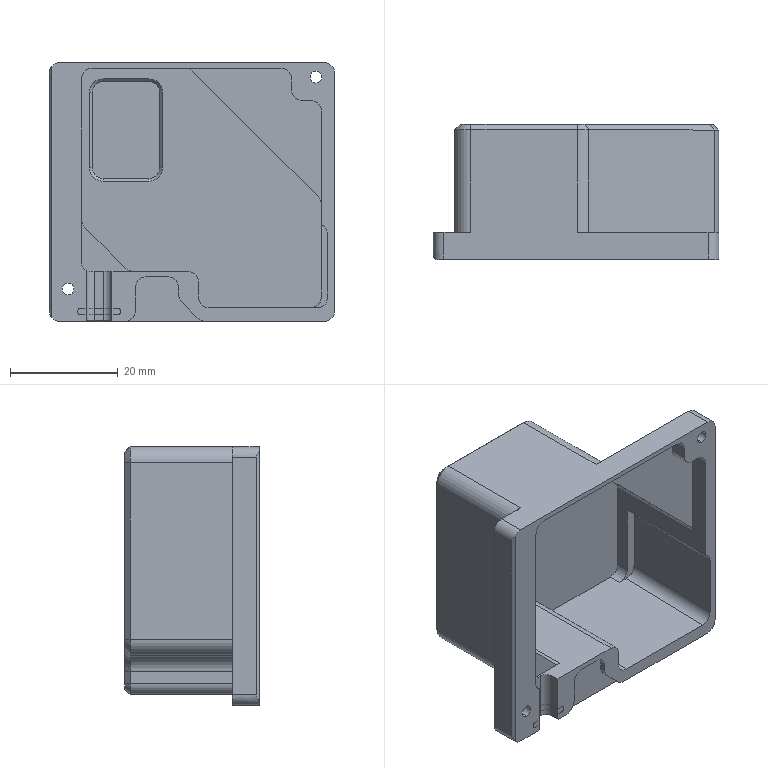NC program | NX | posted with a generic post | part box 53 x 25 x 48 mm
Lines 5523 to 6007 of 6007:
(FLOOR_FACING_1 , TOOL : D4-12-D4-50-3T-FINISH)
N10978 T13 M6
N10980 G54
N10982 G17 G0 G90 X-6.366 Y8.78 B0. C0. S3500 M3
N10984 G43 Z30. H13
N10986 Z-0.3 B-180. C-180.
N10988 G94 G1 Z-3.3 F600.
N10990 X-9.901 Y12.316
N10992 G3 X-11.316 Y12.316 R1.
N10994 G1 X-20.8 Y2.831
N10996 Y16.3
N10998 X-19.
N11000 G3 X-14.8 Y20.5 R4.2
N11002 G1 Y21.8
N11004 X-1.831
N11006 X-11.316 Y12.316
N11008 X-13.437 Y14.437
N11010 X-17.8 Y10.074
N11012 X-18.642 Y8.041
N11014 X-17.8 Y10.074
N11016 Y13.401
N11018 G3 X-12.004 Y18.8 R7.2
N11020 G1 X-9.074
N11022 X-7.041 Y19.642
N11024 X-9.074 Y18.8
N11026 X-13.437 Y14.437
N11028 X-14.144 Y13.73
N11030 G3 X-14.144 Y12.316 R1.
N11032 G1 X-8.487 Y6.659
N11034 Z-0.3
N11036 G0 Z30.
N11038 X29.2 Y-5.243
N11040 Z2.
N11042 G1 Z-1.
N11044 X24.2
N11046 G3 X23.2 Y-6.243 R1.
N11048 G1 Y-8.475
N11050 G3 X22. Y-8.3 R4.2
N11052 G1 X17.95
N11054 Y-4.7
N11056 X18.972
N11058 G3 X21.941 Y-3.47 R4.2
N11060 G1 X23.2 Y-2.211
N11062 Y-6.243
N11064 X21.4
N11066 Y-6.5
N11068 X19.75
N11070 Y-6.449
N11072 G3 X21.4 Y-5.987 R6.
N11074 G1 Y-6.243
N11076 Y-6.5
N11078 X20.657
N11080 G3 X19.657 Y-7.5 R1.
N11082 G1 X29.2
N11084 Z2.
N11086 G0 Z30.
N11088 X5.991 Y-13.155
N11090 Z2.
N11092 G1 Z-1.
N11094 X9.526 Y-16.691
N11096 G3 X10.941 Y-16.691 R1.
N11098 G1 X12.55 Y-15.081
N11100 Y-17.05
N11102 X13.95
N11104 Y-17.549
N11106 G3 X12.865 Y-18.3 R2.2
N11108 G1 X9.331
N11110 X10.941 Y-16.691
N11112 X11.648 Y-15.984
N11114 G3 X11.648 Y-14.569 R1.
N11116 G1 X8.112 Y-11.034
N11118 Z2.
N11120 G0 Z30.
N11122 X5.991 Y-13.155
N11124 Z-0.3
N11126 G1 Z-3.3
N11128 X9.526 Y-16.691
N11130 G3 X10.941 Y-16.691 R1.
N11132 G1 X12.55 Y-15.081
N11134 Y-18.3
N11136 X9.331
N11138 X10.941 Y-16.691
N11140 X11.648 Y-15.984
N11142 G3 X11.648 Y-14.569 R1.
N11144 G1 X8.112 Y-11.034
N11146 Z-0.3
N11148 G0 Z30.
(PLANAR_MILL_7 , TOOL : D4-12-D4-50-3T-FINISH)
N11150 X8.259 Y12.2
N11152 Z-22.
N11154 G1 X6.388 Z-22.098
N11156 X-5.781 Y0.031 Z-23.
N11158 X-2.387 Y-3.363
N11160 X-2.924 Y-3.9
N11162 X-1.85
N11164 Y-2.826
N11166 X-2.387 Y-3.363
N11168 X-4.084 Y-1.666
N11170 X-8.718 Y-6.3
N11172 X0.118
N11174 X0.55 Y-5.868
N11176 Y-0.8
N11178 G2 X1.15 Y3.568 R16.2
N11180 G1 X-4.084 Y-1.666
N11182 X-5.781 Y0.031
N11184 X-11.2 Y-5.388
N11186 Y-8.7
N11188 X1.112
N11190 X2.95 Y-6.862
N11192 Y-0.8
N11194 G2 X9.7 Y11.063 R13.8
N11196 G1 Y12.2
N11198 X6.388
N11200 X-5.781 Y0.031
N11202 X-7.478 Y1.728
N11204 X-13.6 Y-4.394
N11206 Y-11.1
N11208 X2.106
N11210 X5.35 Y-7.856
N11212 Y-0.8
N11214 G2 X12.1 Y9.609 R11.4
N11216 G1 Y14.6
N11218 X5.394
N11220 X-7.478 Y1.728
N11222 X-9.175 Y3.425
N11224 X-16. Y-3.399
N11226 Y-13.5
N11228 X3.101
N11230 X7.75 Y-8.851
N11232 Y-0.8
N11234 G2 X14.5 Y7.914 R9.
N11236 G1 Y17.
N11238 X4.399
N11240 X-9.175 Y3.425
N11242 X-10.872 Y5.122
N11244 X-18.4 Y-2.405
N11246 Y-15.9
N11248 X4.095
N11250 X10.15 Y-9.845
N11252 Y-0.8
N11254 G2 X16.75 Y5.8 R6.6
N11256 G1 X16.9
N11258 Y19.4
N11260 X3.405
N11262 X-10.872 Y5.122
N11264 X-12.569 Y6.819
N11266 X-20.8 Y-1.411
N11268 Y-18.3
N11270 X5.089
N11272 X12.55 Y-10.839
N11274 Y-0.8
N11276 G2 X16.75 Y3.4 R4.2
N11278 G1 X19.3
N11280 Y21.8
N11282 X2.411
N11284 X-12.569 Y6.819
N11286 Z-22.
N11288 G0 Z30.
(FLOOR_FACING_1_COPY , TOOL : D4-12-D4-50-3T-FINISH)
N11290 X-8.481 Y-8.1
N11292 Z-23.
N11294 G1 X-4.6 Z-23.203
N11296 Y-16.4 Z-23.638
N11298 X-11.5 Z-24.
N11300 X-18.4
N11302 Y-8.1
N11304 X-4.6
N11306 Y-16.4
N11308 X-11.5
N11310 Y-13.4
N11312 X-15.4
N11314 Y-11.1
N11316 X-7.6
N11318 Y-13.4
N11320 X-11.5
N11322 X-12.5
N11324 Z-23.
N11326 G0 Z30.
(PLANAR_MILL_7_COPY , TOOL : D4-12-D4-50-3T-FINISH)
N11328 X17.5 Y5.2
N11330 Z-5.66
N11332 G1 Z-7.66
N11334 G3 X19.5 Y3.2 R2.
N11336 G1 Y22.
N11338 X2.328
N11340 X-21. Y-1.328
N11342 Y-18.5
N11344 X5.172
N11346 X12.75 Y-10.922
N11348 Y-0.8
N11350 G2 X16.75 Y3.2 R4.
N11352 G1 X19.5
N11354 G3 X17.5 Y5.2 R2.
N11356 X19.5 Y3.2 R2.
N11358 G1 Y22.
N11360 X2.328
N11362 X-21. Y-1.328
N11364 Y-18.5
N11366 X5.172
N11368 X12.75 Y-10.922
N11370 Y-0.8
N11372 G2 X16.75 Y3.2 R4.
N11374 G1 X19.5
N11376 G3 X17.5 Y5.2 R2.
N11378 G1 Z-5.66
N11380 G0 Z30.
N11382 Z-13.32
N11384 G1 Z-15.32
N11386 G3 X19.5 Y3.2 R2.
N11388 G1 Y22.
N11390 X2.328
N11392 X-21. Y-1.328
N11394 Y-18.5
N11396 X5.172
N11398 X12.75 Y-10.922
N11400 Y-0.8
N11402 G2 X16.75 Y3.2 R4.
N11404 G1 X19.5
N11406 G3 X17.5 Y5.2 R2.
N11408 X19.5 Y3.2 R2.
N11410 G1 Y22.
N11412 X2.328
N11414 X-21. Y-1.328
N11416 Y-18.5
N11418 X5.172
N11420 X12.75 Y-10.922
N11422 Y-0.8
N11424 G2 X16.75 Y3.2 R4.
N11426 G1 X19.5
N11428 G3 X17.5 Y5.2 R2.
N11430 G1 Z-13.32
N11432 G0 Z30.
N11434 Z-20.98
N11436 G1 Z-22.98
N11438 G3 X19.5 Y3.2 R2.
N11440 G1 Y22.
N11442 X2.328
N11444 X-21. Y-1.328
N11446 Y-18.5
N11448 X5.172
N11450 X12.75 Y-10.922
N11452 Y-0.8
N11454 G2 X16.75 Y3.2 R4.
N11456 G1 X19.5
N11458 G3 X17.5 Y5.2 R2.
N11460 X19.5 Y3.2 R2.
N11462 G1 Y22.
N11464 X2.328
N11466 X-21. Y-1.328
N11468 Y-18.5
N11470 X5.172
N11472 X12.75 Y-10.922
N11474 Y-0.8
N11476 G2 X16.75 Y3.2 R4.
N11478 G1 X19.5
N11480 G3 X17.5 Y5.2 R2.
N11482 G1 Z-20.98
N11484 G0 Z30.
(PLANAR_MILL_7_COPY_COPY , TOOL : D4-12-D4-50-3T-FINISH)
N11486 X-6.5 Y-10.
N11488 Z-22.
N11490 G1 Z-24.
N11492 G3 X-4.5 Y-8. R2.
N11494 G1 X-18.5
N11496 Y-16.5
N11498 X-4.5
N11500 Y-8.
N11502 G3 X-6.5 Y-10. R2.
N11504 X-4.5 Y-8. R2.
N11506 G1 X-18.5
N11508 Y-16.5
N11510 X-4.5
N11512 Y-8.
N11514 G3 X-6.5 Y-10. R2.
N11516 G1 Z-22.
N11518 G0 Z30.
(PLANAR_MILL_7_COPY_COPY_COPY , TOOL : D4-12-D4-50-3T-FINISH)
N11520 X4.328 Y20.
N11522 Z-1.3
N11524 G1 Z-3.3
N11526 G3 X2.328 Y22. R2.
N11528 G1 X-15.
N11530 Y20.5
N11532 G2 X-19. Y16.5 R4.
N11534 G1 X-20.95
N11536 Y-1.278
N11538 G3 X-18.95 Y-3.278 R2.
N11540 G1 Z-1.3
N11542 G0 Z30.
N11544 X4.328 Y20.
N11546 Z-1.3
N11548 G1 Z-3.3
N11550 G3 X2.328 Y22. R2.
N11552 G1 X-15.
N11554 Y20.5
N11556 G2 X-19. Y16.5 R4.
N11558 G1 X-20.95
N11560 Y-1.278
N11562 G3 X-18.95 Y-3.278 R2.
N11564 G1 Z-1.3
N11566 G0 Z30.
N11568 X3.172 Y-16.5
N11570 Z-1.3
N11572 G1 Z-3.3
N11574 G3 X5.172 Y-18.5 R2.
N11576 G1 X12.75
N11578 Y-10.922
N11580 G3 X10.75 Y-8.922 R2.
N11582 G1 Z-1.3
N11584 G0 Z30.
N11586 X3.172 Y-16.5
N11588 Z-1.3
N11590 G1 Z-3.3
N11592 G3 X5.172 Y-18.5 R2.
N11594 G1 X12.75
N11596 Y-10.922
N11598 G3 X10.75 Y-8.922 R2.
N11600 G1 Z-1.3
N11602 G0 Z30.
(PLANAR_MILL_7_COPY_COPY_COPY_COPY , TOOL : D4-12-D4-50-3T-FINISH)
N11604 X28. Y4.528
N11606 Z1.
N11608 G1 Z-1.
N11610 G3 X26. Y2.528 R2.
N11612 G2 X24.828 Y-0.3 R4.
N11614 G1 X21.8 Y-3.328
N11616 G2 X18.972 Y-4.5 R4.
N11618 G1 X17.75
N11620 Y-8.5
N11622 X22.
N11624 G2 X26. Y-12.5 R4.
N11626 G3 X28. Y-14.5 R2.
N11628 G1 Z1.
N11630 G0 Z30.
N11632 Y4.528
N11634 Z1.
N11636 G1 Z-1.
N11638 G3 X26. Y2.528 R2.
N11640 G2 X24.828 Y-0.3 R4.
N11642 G1 X21.8 Y-3.328
N11644 G2 X18.972 Y-4.5 R4.
N11646 G1 X17.75
N11648 Y-8.5
N11650 X22.
N11652 G2 X26. Y-12.5 R4.
N11654 G3 X28. Y-14.5 R2.
N11656 G1 Z1.
N11658 G0 Z30.
N11660 M5
(PLANAR_MILL_8 , TOOL : 倒角D3-90度)
N11662 T14 M6
N11664 G54
N11666 G17 G0 G90 X27. Y-17.85 B0. C0. S3500 M3
N11668 G43 Z30. H14
N11670 Z1. B-180. C-180.
N11672 G94 G1 Z-1. F800.
N11674 G3 X25. Y-19.85 R2.
N11676 G1 Y-24.5
N11678 G2 X23.984 Y-26.75 R3.
N11680 X23.323 Y-27. R1.
N11682 G1 X-23.323
N11684 G2 X-23.984 Y-26.75 R1.
N11686 X-25. Y-24.5 R3.
N11688 G1 Y24.5
N11690 G2 X-22. Y27.5 R3.
N11692 G1 X22.
N11694 G2 X25. Y24.5 R3.
N11696 G1 Y2.528
N11698 G2 X24.121 Y0.407 R3.
N11700 G1 X21.093 Y-2.621
N11702 G2 X18.972 Y-3.5 R3.
N11704 G1 X17.75
N11706 G3 X16.75 Y-4.5 R1.
N11708 G1 Y-8.5
N11710 G3 X17.75 Y-9.5 R1.
N11712 G1 X22.
N11714 G2 X25. Y-12.5 R3.
N11716 G1 Y-14.65
N11718 G3 X27. Y-16.65 R2.
N11720 G1 Z1.
N11722 G0 Z30.
(PLANAR_MILL_8_COPY , TOOL : 倒角D3-90度)
N11724 X22.6 Y-16.85
N11726 Z1.
N11728 G1 Z-1.
N11730 G3 X21.6 Y-15.85 R1.
N11732 G1 X14.75
N11734 G2 X13.75 Y-14.85 R1.
N11736 G1 Y-0.8
N11738 G2 X16.75 Y2.2 R3.
N11740 G1 X19.5
N11742 G3 X20.5 Y3.2 R1.
N11744 G1 Y23.199
N11746 X20.489 Y23.344
N11748 G3 X20.154 Y23.957 R1.001
N11750 X19.5 Y24.2 R0.999
N11752 G1 X7.833
N11754 G3 X7.286 Y24.037 R1.
N11756 X6.916 Y23.6 R1.002
N11758 G2 X6. Y23. R1.
N11760 G1 X-15.
N11762 G3 X-16. Y22. R1.
N11764 G1 Y20.5
N11766 G2 X-19. Y17.5 R3.
N11768 G1 X-21.
N11770 G3 X-22. Y16.5 R1.
N11772 G1 Y-18.5
N11774 G3 X-21. Y-19.5 R1.
N11776 G1 X13.25
N11778 G3 X13.701 Y-19.217 R0.5
N11780 G2 X14.602 Y-18.65 R1.
N11782 G1 X21.6
N11784 G3 X22.6 Y-17.65 R1.
N11786 G1 Z1.
N11788 G0 Z30.
(PLANAR_MILL_8_COPY_COPY , TOOL : 倒角D3-90度)
N11790 X1.769 Y21.158
N11792 Z-2.5
N11794 G1 Z-4.5
N11796 G3 X0.355 Y21.158 R1.
N11798 G1 X-20.158 Y0.645
N11800 G3 X-20.158 Y-0.769 R1.
N11802 G1 Z-2.5
N11804 G0 Z30.
N11806 X5.538 Y-17.851
N11808 Z-2.5
N11810 G1 Z-4.5
N11812 G3 X6.952 Y-17.851 R1.
N11814 G1 X12.101 Y-12.702
N11816 G3 X12.101 Y-11.288 R1.
N11818 G1 Z-2.5
N11820 G0 Z30.
(PLANAR_MILL_8_COPY_COPY_COPY , TOOL : 倒角D3-90度)
N11822 X-10.5 Y-7.5
N11824 Z-22.
N11826 G1 Z-24.
N11828 G3 X-11.5 Y-6.5 R1.
N11830 G1 X-18.5
N11832 G3 X-20. Y-8. R1.5
N11834 G1 Y-16.5
N11836 G3 X-18.5 Y-18. R1.5
N11838 G1 X-4.5
N11840 G3 X-3. Y-16.5 R1.5
N11842 G1 Y-8.
N11844 G3 X-4.5 Y-6.5 R1.5
N11846 G1 X-11.5
N11848 G3 X-12.5 Y-7.5 R1.
N11850 G1 X-10.5
N11852 G3 X-11.5 Y-6.5 R1.
N11854 G1 X-18.5
N11856 G3 X-20. Y-8. R1.5
N11858 G1 Y-16.5
N11860 G3 X-18.5 Y-18. R1.5
N11862 G1 X-4.5
N11864 G3 X-3. Y-16.5 R1.5
N11866 G1 Y-8.
N11868 G3 X-4.5 Y-6.5 R1.5
N11870 G1 X-11.5
N11872 G3 X-12.5 Y-7.5 R1.
N11874 G1 Z-22.
N11876 G0 Z30.
N11878 M5
N11880 M2